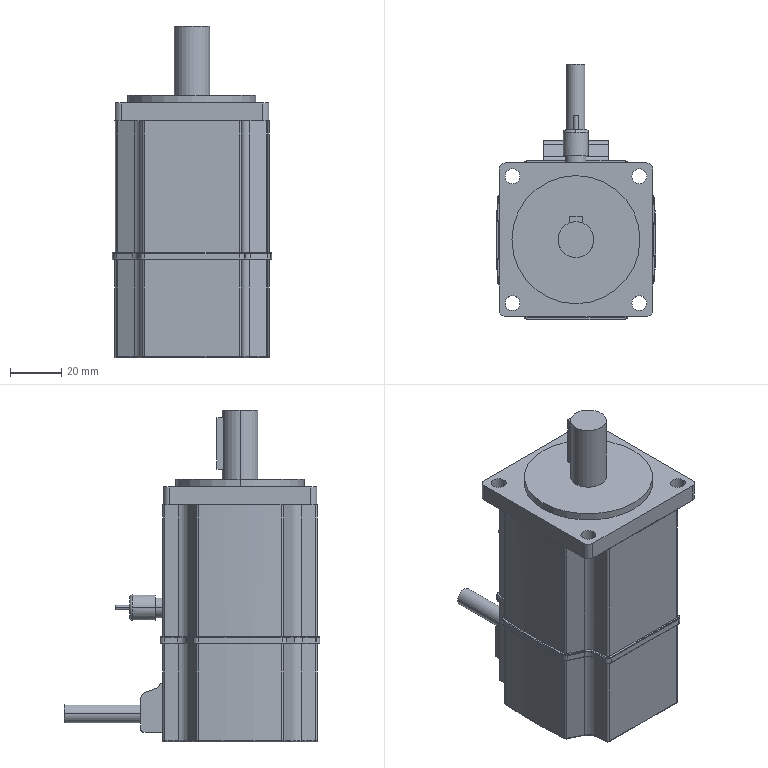Part | STEP file | 2 solids | 255 faces | box 62.422 x 99.9 x 129.5 mm | volume 546623 mm3 | cylinder 131 | torus 57 | plane 53 | sphere 10 | spline 4 | commonest cylinder face diameters 0.5 x36 2 x16 1 x12 4 x10 5.8 x8 10 x8